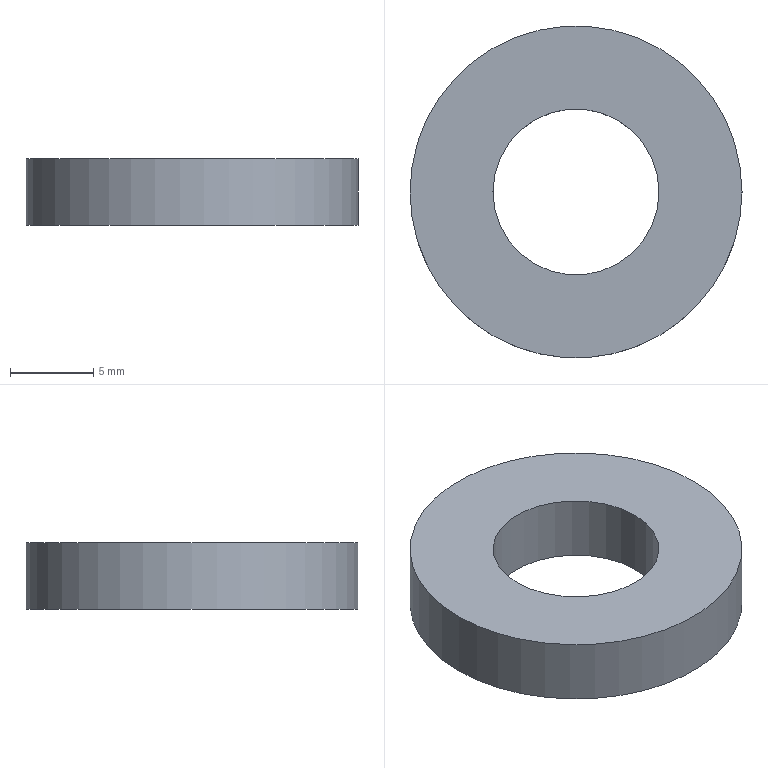Part | STEP file | YBQDJ-YB-33 | 1 solid | 4 faces | box 20 x 20 x 4 mm | volume 942.478 mm3 | plane 2 | cylinder 2 | commonest cylinder face diameters 10 x1 20 x1
STEP:
#1=CARTESIAN_POINT('',(0.,0.,0.));
#2=DIRECTION('',(0.,0.,1.));
#3=DIRECTION('',(1.,0.,0.));
#4=AXIS2_PLACEMENT_3D('',#1,#2,#3);
#5=CARTESIAN_POINT('',(-281.5,-281.,136.2));
#6=VERTEX_POINT('',#5);
#7=CARTESIAN_POINT('',(-271.5,-281.,136.2));
#8=DIRECTION('',(0.,0.,1.));
#9=DIRECTION('',(-1.,0.,0.));
#10=AXIS2_PLACEMENT_3D('',#7,#8,#9);
#11=CIRCLE('',#10,10.);
#12=CARTESIAN_POINT('',(-271.5,-281.,136.2));
#13=DIRECTION('',(0.,0.,-1.));
#14=DIRECTION('',(-1.,0.,0.));
#15=AXIS2_PLACEMENT_3D('',#12,#13,#14);
#16=PLANE('',#15);
#17=CARTESIAN_POINT('',(10.,0.));
#18=CARTESIAN_POINT('',(10.,-17.321));
#19=CARTESIAN_POINT('',(-5.,-8.66));
#20=CARTESIAN_POINT('',(-20.,0.));
#21=CARTESIAN_POINT('',(-5.,8.66));
#22=CARTESIAN_POINT('',(10.,17.321));
#23=CARTESIAN_POINT('',(10.,0.));
#24=(BOUNDED_CURVE()B_SPLINE_CURVE(2,(#17,#18,#19,#20,#21,#22,#23),.UNSPECIFIED.,.T.,.F.)B_SPLINE_CURVE_WITH_KNOTS((1,2,2,2,2,1),(-2.094,0.,2.094,4.189,6.283,8.378),.UNSPECIFIED.)CURVE()GEOMETRIC_REPRESENTATION_ITEM()RATIONAL_B_SPLINE_CURVE((1.,0.5,1.,0.5,1.,0.5,1.))REPRESENTATION_ITEM(''));
#25=(GEOMETRIC_REPRESENTATION_CONTEXT(2)PARAMETRIC_REPRESENTATION_CONTEXT()REPRESENTATION_CONTEXT('',''));
#26=DEFINITIONAL_REPRESENTATION('',(#24),#25);
#27=PCURVE('',#16,#26);
#28=CARTESIAN_POINT('',(-271.5,-281.,136.2));
#29=DIRECTION('',(0.,0.,1.));
#30=DIRECTION('',(1.,0.,0.));
#31=AXIS2_PLACEMENT_3D('',#28,#29,#30);
#32=CYLINDRICAL_SURFACE('',#31,10.);
#33=CARTESIAN_POINT('',(3.142,0.));
#34=DIRECTION('',(1.,0.));
#35=VECTOR('',#34,1.);
#36=LINE('',#33,#35);
#37=(GEOMETRIC_REPRESENTATION_CONTEXT(2)PARAMETRIC_REPRESENTATION_CONTEXT()REPRESENTATION_CONTEXT('',''));
#38=DEFINITIONAL_REPRESENTATION('',(#36),#37);
#39=PCURVE('',#32,#38);
#40=SURFACE_CURVE('',#11,(#27,#39),.PCURVE_S1.);
#41=EDGE_CURVE('',#6,#6,#40,.T.);
#42=ORIENTED_EDGE('',*,*,#41,.F.);
#43=EDGE_LOOP('',(#42));
#44=FACE_BOUND('',#43,.T.);
#45=CARTESIAN_POINT('',(-266.5,-281.,136.2));
#46=VERTEX_POINT('',#45);
#47=CARTESIAN_POINT('',(-271.5,-281.,136.2));
#48=DIRECTION('',(0.,0.,1.));
#49=DIRECTION('',(1.,0.,0.));
#50=AXIS2_PLACEMENT_3D('',#47,#48,#49);
#51=CIRCLE('',#50,5.);
#52=CARTESIAN_POINT('',(-5.,0.));
#53=CARTESIAN_POINT('',(-5.,8.66));
#54=CARTESIAN_POINT('',(2.5,4.33));
#55=CARTESIAN_POINT('',(10.,0.));
#56=CARTESIAN_POINT('',(2.5,-4.33));
#57=CARTESIAN_POINT('',(-5.,-8.66));
#58=CARTESIAN_POINT('',(-5.,0.));
#59=(BOUNDED_CURVE()B_SPLINE_CURVE(2,(#52,#53,#54,#55,#56,#57,#58),.UNSPECIFIED.,.T.,.F.)B_SPLINE_CURVE_WITH_KNOTS((1,2,2,2,2,1),(-2.094,0.,2.094,4.189,6.283,8.378),.UNSPECIFIED.)CURVE()GEOMETRIC_REPRESENTATION_ITEM()RATIONAL_B_SPLINE_CURVE((1.,0.5,1.,0.5,1.,0.5,1.))REPRESENTATION_ITEM(''));
#60=(GEOMETRIC_REPRESENTATION_CONTEXT(2)PARAMETRIC_REPRESENTATION_CONTEXT()REPRESENTATION_CONTEXT('',''));
#61=DEFINITIONAL_REPRESENTATION('',(#59),#60);
#62=PCURVE('',#16,#61);
#63=CARTESIAN_POINT('',(-271.5,-281.,136.2));
#64=DIRECTION('',(0.,0.,1.));
#65=DIRECTION('',(1.,0.,0.));
#66=AXIS2_PLACEMENT_3D('',#63,#64,#65);
#67=CYLINDRICAL_SURFACE('',#66,5.);
#68=CARTESIAN_POINT('',(0.,0.));
#69=DIRECTION('',(1.,0.));
#70=VECTOR('',#69,1.);
#71=LINE('',#68,#70);
#72=(GEOMETRIC_REPRESENTATION_CONTEXT(2)PARAMETRIC_REPRESENTATION_CONTEXT()REPRESENTATION_CONTEXT('',''));
#73=DEFINITIONAL_REPRESENTATION('',(#71),#72);
#74=PCURVE('',#67,#73);
#75=SURFACE_CURVE('',#51,(#62,#74),.PCURVE_S1.);
#76=EDGE_CURVE('',#46,#46,#75,.T.);
#77=ORIENTED_EDGE('',*,*,#76,.T.);
#78=EDGE_LOOP('',(#77));
#79=FACE_BOUND('',#78,.T.);
#80=ADVANCED_FACE('',(#44,#79),#16,.T.);
#81=CARTESIAN_POINT('',(-281.5,-281.,140.2));
#82=VERTEX_POINT('',#81);
#83=CARTESIAN_POINT('',(-271.5,-281.,140.2));
#84=DIRECTION('',(0.,0.,1.));
#85=DIRECTION('',(-1.,0.,0.));
#86=AXIS2_PLACEMENT_3D('',#83,#84,#85);
#87=CIRCLE('',#86,10.);
#88=CARTESIAN_POINT('',(-271.5,-281.,140.2));
#89=DIRECTION('',(0.,0.,-1.));
#90=DIRECTION('',(-1.,0.,0.));
#91=AXIS2_PLACEMENT_3D('',#88,#89,#90);
#92=PLANE('',#91);
#93=CARTESIAN_POINT('',(10.,0.));
#94=CARTESIAN_POINT('',(10.,-17.321));
#95=CARTESIAN_POINT('',(-5.,-8.66));
#96=CARTESIAN_POINT('',(-20.,0.));
#97=CARTESIAN_POINT('',(-5.,8.66));
#98=CARTESIAN_POINT('',(10.,17.321));
#99=CARTESIAN_POINT('',(10.,0.));
#100=(BOUNDED_CURVE()B_SPLINE_CURVE(2,(#93,#94,#95,#96,#97,#98,#99),.UNSPECIFIED.,.T.,.F.)B_SPLINE_CURVE_WITH_KNOTS((1,2,2,2,2,1),(-2.094,0.,2.094,4.189,6.283,8.378),.UNSPECIFIED.)CURVE()GEOMETRIC_REPRESENTATION_ITEM()RATIONAL_B_SPLINE_CURVE((1.,0.5,1.,0.5,1.,0.5,1.))REPRESENTATION_ITEM(''));
#101=(GEOMETRIC_REPRESENTATION_CONTEXT(2)PARAMETRIC_REPRESENTATION_CONTEXT()REPRESENTATION_CONTEXT('',''));
#102=DEFINITIONAL_REPRESENTATION('',(#100),#101);
#103=PCURVE('',#92,#102);
#104=CARTESIAN_POINT('',(3.142,4.));
#105=DIRECTION('',(1.,0.));
#106=VECTOR('',#105,1.);
#107=LINE('',#104,#106);
#108=(GEOMETRIC_REPRESENTATION_CONTEXT(2)PARAMETRIC_REPRESENTATION_CONTEXT()REPRESENTATION_CONTEXT('',''));
#109=DEFINITIONAL_REPRESENTATION('',(#107),#108);
#110=PCURVE('',#32,#109);
#111=SURFACE_CURVE('',#87,(#103,#110),.PCURVE_S1.);
#112=EDGE_CURVE('',#82,#82,#111,.T.);
#113=ORIENTED_EDGE('',*,*,#112,.T.);
#114=EDGE_LOOP('',(#113));
#115=FACE_BOUND('',#114,.T.);
#116=CARTESIAN_POINT('',(-276.5,-281.,140.2));
#117=VERTEX_POINT('',#116);
#118=CARTESIAN_POINT('',(-266.5,-281.,140.2));
#119=VERTEX_POINT('',#118);
#120=CARTESIAN_POINT('',(-271.5,-281.,140.2));
#121=DIRECTION('',(0.,0.,1.));
#122=DIRECTION('',(-1.,0.,0.));
#123=AXIS2_PLACEMENT_3D('',#120,#121,#122);
#124=CIRCLE('',#123,5.);
#125=CARTESIAN_POINT('',(5.,0.));
#126=CARTESIAN_POINT('',(5.,-8.66));
#127=CARTESIAN_POINT('',(-2.5,-4.33));
#128=CARTESIAN_POINT('',(-10.,0.));
#129=CARTESIAN_POINT('',(-2.5,4.33));
#130=CARTESIAN_POINT('',(5.,8.66));
#131=CARTESIAN_POINT('',(5.,0.));
#132=(BOUNDED_CURVE()B_SPLINE_CURVE(2,(#125,#126,#127,#128,#129,#130,#131),.UNSPECIFIED.,.T.,.F.)B_SPLINE_CURVE_WITH_KNOTS((1,2,2,2,2,1),(-2.094,0.,2.094,4.189,6.283,8.378),.UNSPECIFIED.)CURVE()GEOMETRIC_REPRESENTATION_ITEM()RATIONAL_B_SPLINE_CURVE((1.,0.5,1.,0.5,1.,0.5,1.))REPRESENTATION_ITEM(''));
#133=(GEOMETRIC_REPRESENTATION_CONTEXT(2)PARAMETRIC_REPRESENTATION_CONTEXT()REPRESENTATION_CONTEXT('',''));
#134=DEFINITIONAL_REPRESENTATION('',(#132),#133);
#135=PCURVE('',#92,#134);
#136=CARTESIAN_POINT('',(3.142,4.));
#137=DIRECTION('',(1.,0.));
#138=VECTOR('',#137,1.);
#139=LINE('',#136,#138);
#140=(GEOMETRIC_REPRESENTATION_CONTEXT(2)PARAMETRIC_REPRESENTATION_CONTEXT()REPRESENTATION_CONTEXT('',''));
#141=DEFINITIONAL_REPRESENTATION('',(#139),#140);
#142=PCURVE('',#67,#141);
#143=SURFACE_CURVE('',#124,(#135,#142),.PCURVE_S1.);
#144=EDGE_CURVE('',#117,#119,#143,.T.);
#145=ORIENTED_EDGE('',*,*,#144,.F.);
#146=CARTESIAN_POINT('',(-271.5,-281.,140.2));
#147=DIRECTION('',(0.,0.,1.));
#148=DIRECTION('',(-1.,0.,0.));
#149=AXIS2_PLACEMENT_3D('',#146,#147,#148);
#150=CIRCLE('',#149,5.);
#151=CARTESIAN_POINT('',(5.,0.));
#152=CARTESIAN_POINT('',(5.,-8.66));
#153=CARTESIAN_POINT('',(-2.5,-4.33));
#154=CARTESIAN_POINT('',(-10.,0.));
#155=CARTESIAN_POINT('',(-2.5,4.33));
#156=CARTESIAN_POINT('',(5.,8.66));
#157=CARTESIAN_POINT('',(5.,0.));
#158=(BOUNDED_CURVE()B_SPLINE_CURVE(2,(#151,#152,#153,#154,#155,#156,#157),.UNSPECIFIED.,.T.,.F.)B_SPLINE_CURVE_WITH_KNOTS((1,2,2,2,2,1),(-2.094,0.,2.094,4.189,6.283,8.378),.UNSPECIFIED.)CURVE()GEOMETRIC_REPRESENTATION_ITEM()RATIONAL_B_SPLINE_CURVE((1.,0.5,1.,0.5,1.,0.5,1.))REPRESENTATION_ITEM(''));
#159=(GEOMETRIC_REPRESENTATION_CONTEXT(2)PARAMETRIC_REPRESENTATION_CONTEXT()REPRESENTATION_CONTEXT('',''));
#160=DEFINITIONAL_REPRESENTATION('',(#158),#159);
#161=PCURVE('',#92,#160);
#162=CARTESIAN_POINT('',(-3.142,4.));
#163=DIRECTION('',(1.,0.));
#164=VECTOR('',#163,1.);
#165=LINE('',#162,#164);
#166=(GEOMETRIC_REPRESENTATION_CONTEXT(2)PARAMETRIC_REPRESENTATION_CONTEXT()REPRESENTATION_CONTEXT('',''));
#167=DEFINITIONAL_REPRESENTATION('',(#165),#166);
#168=PCURVE('',#67,#167);
#169=SURFACE_CURVE('',#150,(#161,#168),.PCURVE_S1.);
#170=EDGE_CURVE('',#119,#117,#169,.T.);
#171=ORIENTED_EDGE('',*,*,#170,.F.);
#172=EDGE_LOOP('',(#145,#171));
#173=FACE_BOUND('',#172,.T.);
#174=ADVANCED_FACE('',(#115,#173),#92,.F.);
#175=ORIENTED_EDGE('',*,*,#41,.T.);
#176=CARTESIAN_POINT('',(-281.5,-281.,136.2));
#177=CARTESIAN_POINT('',(-281.5,-281.,140.2));
#178=B_SPLINE_CURVE_WITH_KNOTS('',1,(#176,#177),.UNSPECIFIED.,.F.,.F.,(2,2),(0.,4.),.PIECEWISE_BEZIER_KNOTS.);
#179=CARTESIAN_POINT('',(9.425,0.));
#180=DIRECTION('',(0.,1.));
#181=VECTOR('',#180,1.);
#182=LINE('',#179,#181);
#183=(GEOMETRIC_REPRESENTATION_CONTEXT(2)PARAMETRIC_REPRESENTATION_CONTEXT()REPRESENTATION_CONTEXT('',''));
#184=DEFINITIONAL_REPRESENTATION('',(#182),#183);
#185=PCURVE('',#32,#184);
#186=CARTESIAN_POINT('',(3.142,0.));
#187=DIRECTION('',(0.,1.));
#188=VECTOR('',#187,1.);
#189=LINE('',#186,#188);
#190=(GEOMETRIC_REPRESENTATION_CONTEXT(2)PARAMETRIC_REPRESENTATION_CONTEXT()REPRESENTATION_CONTEXT('',''));
#191=DEFINITIONAL_REPRESENTATION('',(#189),#190);
#192=PCURVE('',#32,#191);
#193=SEAM_CURVE('',#178,(#185,#192),.PCURVE_S1.);
#194=EDGE_CURVE('',#6,#82,#193,.T.);
#195=ORIENTED_EDGE('',*,*,#194,.T.);
#196=ORIENTED_EDGE('',*,*,#112,.F.);
#197=ORIENTED_EDGE('',*,*,#194,.F.);
#198=EDGE_LOOP('',(#175,#195,#196,#197));
#199=FACE_BOUND('',#198,.T.);
#200=ADVANCED_FACE('',(#199),#32,.T.);
#201=ORIENTED_EDGE('',*,*,#76,.T.);
#202=CARTESIAN_POINT('',(-266.5,-281.,136.2));
#203=CARTESIAN_POINT('',(-266.5,-281.,140.2));
#204=B_SPLINE_CURVE_WITH_KNOTS('',1,(#202,#203),.UNSPECIFIED.,.F.,.F.,(2,2),(0.,4.),.PIECEWISE_BEZIER_KNOTS.);
#205=CARTESIAN_POINT('',(6.283,0.));
#206=DIRECTION('',(0.,1.));
#207=VECTOR('',#206,1.);
#208=LINE('',#205,#207);
#209=(GEOMETRIC_REPRESENTATION_CONTEXT(2)PARAMETRIC_REPRESENTATION_CONTEXT()REPRESENTATION_CONTEXT('',''));
#210=DEFINITIONAL_REPRESENTATION('',(#208),#209);
#211=PCURVE('',#67,#210);
#212=CARTESIAN_POINT('',(0.,0.));
#213=DIRECTION('',(0.,1.));
#214=VECTOR('',#213,1.);
#215=LINE('',#212,#214);
#216=(GEOMETRIC_REPRESENTATION_CONTEXT(2)PARAMETRIC_REPRESENTATION_CONTEXT()REPRESENTATION_CONTEXT('',''));
#217=DEFINITIONAL_REPRESENTATION('',(#215),#216);
#218=PCURVE('',#67,#217);
#219=SEAM_CURVE('',#204,(#211,#218),.PCURVE_S1.);
#220=EDGE_CURVE('',#46,#119,#219,.T.);
#221=ORIENTED_EDGE('',*,*,#220,.T.);
#222=ORIENTED_EDGE('',*,*,#144,.F.);
#223=ORIENTED_EDGE('',*,*,#170,.F.);
#224=ORIENTED_EDGE('',*,*,#220,.F.);
#225=EDGE_LOOP('',(#201,#221,#222,#223,#224));
#226=FACE_BOUND('',#225,.F.);
#227=ADVANCED_FACE('',(#226),#67,.F.);
#228=CLOSED_SHELL('',(#80,#174,#200,#227));
#229=MANIFOLD_SOLID_BREP('',#228);
#230=(LENGTH_UNIT()NAMED_UNIT(*)SI_UNIT(.MILLI.,.METRE.));
#231=UNCERTAINTY_MEASURE_WITH_UNIT(LENGTH_MEASURE(0.000005),#230,'','');
#232=(NAMED_UNIT(*)PLANE_ANGLE_UNIT()SI_UNIT($,.RADIAN.));
#233=(NAMED_UNIT(*)SI_UNIT($,.STERADIAN.)SOLID_ANGLE_UNIT());
#234=(GEOMETRIC_REPRESENTATION_CONTEXT(3)GLOBAL_UNCERTAINTY_ASSIGNED_CONTEXT((#231))GLOBAL_UNIT_ASSIGNED_CONTEXT((#230,#232,#233))REPRESENTATION_CONTEXT('',''));
#235=ADVANCED_BREP_SHAPE_REPRESENTATION('',(#4,#229),#234);